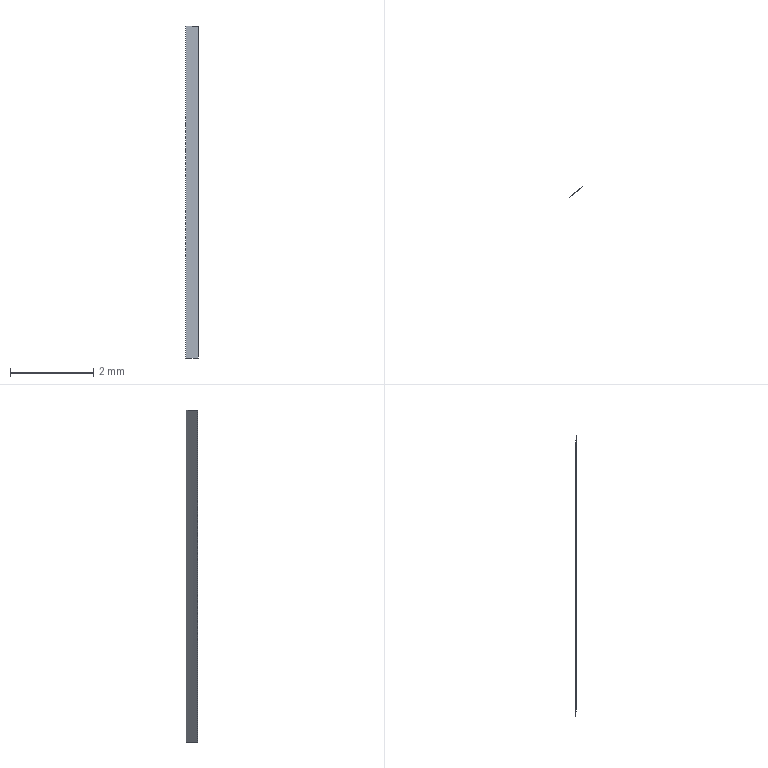Part | STEP file | lll_id198_x_t | 1 solid | 2 faces | box 0.2957 x 0.2677 x 8 mm | volume 0.00006891 mm3 | other 2